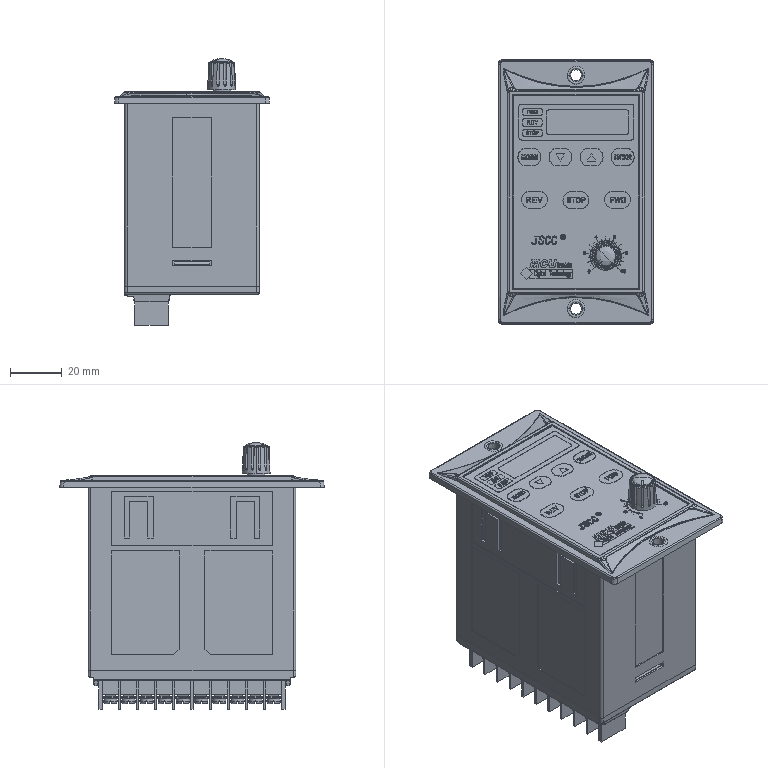Part | SolidWorks | features BaseBody 1 | 1 solid | 2594 faces | box 60 x 102 x 102.7 mm | volume 330811 mm3 | plane 1711 | spline 453 | cylinder 308 | torus 62 | sphere 41 | cone 19 | commonest cylinder face diameters 1 x120 0.6 x65 0.4 x48 5.2 x20 12.166 x19 2 x8